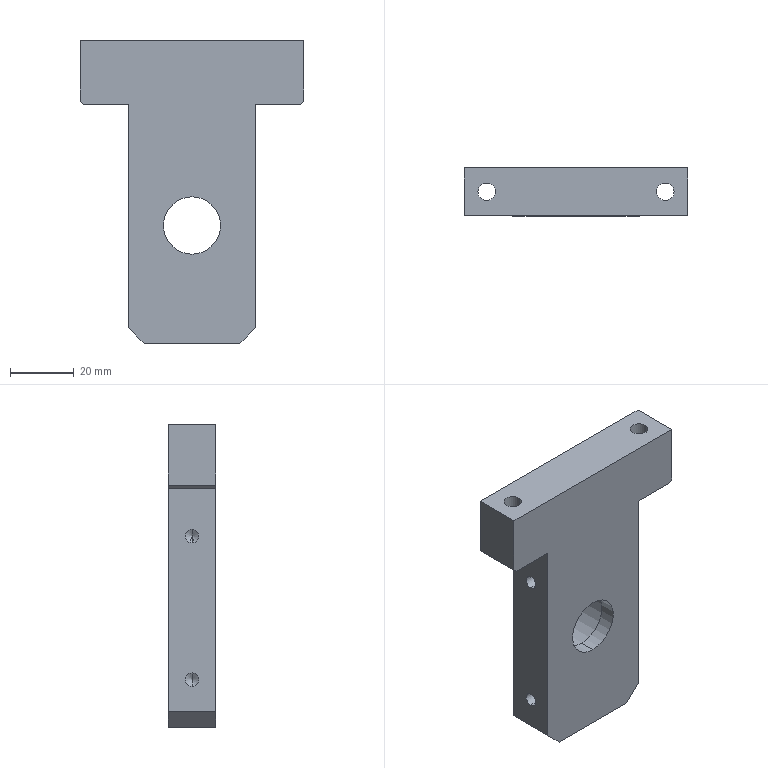Part | SolidWorks | features BaseBody 1 | 1 solid | 45 faces | box 70 x 15 x 95 mm | volume 57528 mm3 | cylinder 20 | plane 17 | cone 8 | commonest cylinder face diameters 4.2 x8 5.5 x4 10 x4 18 x2 24 x2
STEP:
#1=CARTESIAN_POINT('',(-10.345,7.5,-15.013));
#2=VERTEX_POINT('',#1);
#3=CARTESIAN_POINT('',(-10.345,7.5,-10.813));
#4=VERTEX_POINT('',#3);
#5=CARTESIAN_POINT('',(-10.345,7.5,-12.913));
#6=DIRECTION('',(-1.,0.,0.));
#7=DIRECTION('',(0.,0.,1.));
#8=AXIS2_PLACEMENT_3D('',#5,#6,#7);
#9=CIRCLE('',#8,2.1);
#10=EDGE_CURVE('',#2,#4,#9,.T.);
#11=ORIENTED_EDGE('',*,*,#10,.F.);
#12=CARTESIAN_POINT('',(-22.745,7.5,-15.013));
#13=VERTEX_POINT('',#12);
#14=CARTESIAN_POINT('',(-22.745,7.5,-15.013));
#15=DIRECTION('',(-1.,0.,0.));
#16=VECTOR('',#15,1000.);
#17=LINE('',#14,#16);
#18=EDGE_CURVE('',#2,#13,#17,.T.);
#19=ORIENTED_EDGE('',*,*,#18,.T.);
#20=CARTESIAN_POINT('',(-22.745,7.5,-10.813));
#21=VERTEX_POINT('',#20);
#22=CARTESIAN_POINT('',(-22.745,7.5,-12.913));
#23=DIRECTION('',(-1.,0.,0.));
#24=DIRECTION('',(0.,0.,1.));
#25=AXIS2_PLACEMENT_3D('',#22,#23,#24);
#26=CIRCLE('',#25,2.1);
#27=EDGE_CURVE('',#13,#21,#26,.T.);
#28=ORIENTED_EDGE('',*,*,#27,.T.);
#29=CARTESIAN_POINT('',(-22.745,7.5,-10.813));
#30=DIRECTION('',(-1.,0.,0.));
#31=VECTOR('',#30,1000.);
#32=LINE('',#29,#31);
#33=EDGE_CURVE('',#4,#21,#32,.T.);
#34=ORIENTED_EDGE('',*,*,#33,.F.);
#35=EDGE_LOOP('',(#11,#19,#28,#34));
#36=FACE_OUTER_BOUND('',#35,.T.);
#37=CARTESIAN_POINT('',(-22.745,7.5,-12.913));
#38=DIRECTION('',(-1.,0.,0.));
#39=DIRECTION('',(0.,0.,1.));
#40=AXIS2_PLACEMENT_3D('',#37,#38,#39);
#41=CYLINDRICAL_SURFACE('',#40,2.1);
#42=ADVANCED_FACE('',(#36),#41,.F.);
#43=CARTESIAN_POINT('',(-9.083,7.5,-12.913));
#44=VERTEX_POINT('',#43);
#45=CARTESIAN_POINT('',(-10.345,7.5,-10.813));
#46=DIRECTION('',(-0.515,0.,0.8572));
#47=VECTOR('',#46,1000.);
#48=LINE('',#45,#47);
#49=EDGE_CURVE('',#44,#4,#48,.T.);
#50=ORIENTED_EDGE('',*,*,#49,.F.);
#51=CARTESIAN_POINT('',(-10.345,7.5,-15.013));
#52=DIRECTION('',(-0.515,0.,-0.8572));
#53=VECTOR('',#52,1000.);
#54=LINE('',#51,#53);
#55=EDGE_CURVE('',#44,#2,#54,.T.);
#56=ORIENTED_EDGE('',*,*,#55,.T.);
#57=ORIENTED_EDGE('',*,*,#10,.T.);
#58=EDGE_LOOP('',(#50,#56,#57));
#59=FACE_OUTER_BOUND('',#58,.T.);
#60=CARTESIAN_POINT('',(-10.345,7.5,-12.913));
#61=DIRECTION('',(-1.,0.,0.));
#62=DIRECTION('',(0.,0.,1.));
#63=AXIS2_PLACEMENT_3D('',#60,#61,#62);
#64=CONICAL_SURFACE('',#63,2.1,1.03);
#65=ADVANCED_FACE('',(#59),#64,.F.);
#66=CARTESIAN_POINT('',(-10.345,7.5,29.987));
#67=VERTEX_POINT('',#66);
#68=CARTESIAN_POINT('',(-10.345,7.5,34.187));
#69=VERTEX_POINT('',#68);
#70=CARTESIAN_POINT('',(-10.345,7.5,32.087));
#71=DIRECTION('',(-1.,0.,0.));
#72=DIRECTION('',(0.,0.,1.));
#73=AXIS2_PLACEMENT_3D('',#70,#71,#72);
#74=CIRCLE('',#73,2.1);
#75=EDGE_CURVE('',#67,#69,#74,.T.);
#76=ORIENTED_EDGE('',*,*,#75,.F.);
#77=CARTESIAN_POINT('',(-22.745,7.5,29.987));
#78=VERTEX_POINT('',#77);
#79=CARTESIAN_POINT('',(-22.745,7.5,29.987));
#80=DIRECTION('',(-1.,0.,0.));
#81=VECTOR('',#80,1000.);
#82=LINE('',#79,#81);
#83=EDGE_CURVE('',#67,#78,#82,.T.);
#84=ORIENTED_EDGE('',*,*,#83,.T.);
#85=CARTESIAN_POINT('',(-22.745,7.5,34.187));
#86=VERTEX_POINT('',#85);
#87=CARTESIAN_POINT('',(-22.745,7.5,32.087));
#88=DIRECTION('',(-1.,0.,0.));
#89=DIRECTION('',(0.,0.,1.));
#90=AXIS2_PLACEMENT_3D('',#87,#88,#89);
#91=CIRCLE('',#90,2.1);
#92=EDGE_CURVE('',#78,#86,#91,.T.);
#93=ORIENTED_EDGE('',*,*,#92,.T.);
#94=CARTESIAN_POINT('',(-22.745,7.5,34.187));
#95=DIRECTION('',(-1.,0.,0.));
#96=VECTOR('',#95,1000.);
#97=LINE('',#94,#96);
#98=EDGE_CURVE('',#69,#86,#97,.T.);
#99=ORIENTED_EDGE('',*,*,#98,.F.);
#100=EDGE_LOOP('',(#76,#84,#93,#99));
#101=FACE_OUTER_BOUND('',#100,.T.);
#102=CARTESIAN_POINT('',(-22.745,7.5,32.087));
#103=DIRECTION('',(-1.,0.,0.));
#104=DIRECTION('',(0.,0.,1.));
#105=AXIS2_PLACEMENT_3D('',#102,#103,#104);
#106=CYLINDRICAL_SURFACE('',#105,2.1);
#107=ADVANCED_FACE('',(#101),#106,.F.);
#108=CARTESIAN_POINT('',(-9.083,7.5,32.087));
#109=VERTEX_POINT('',#108);
#110=CARTESIAN_POINT('',(-10.345,7.5,34.187));
#111=DIRECTION('',(-0.515,0.,0.8572));
#112=VECTOR('',#111,1000.);
#113=LINE('',#110,#112);
#114=EDGE_CURVE('',#109,#69,#113,.T.);
#115=ORIENTED_EDGE('',*,*,#114,.F.);
#116=CARTESIAN_POINT('',(-10.345,7.5,29.987));
#117=DIRECTION('',(-0.515,0.,-0.8572));
#118=VECTOR('',#117,1000.);
#119=LINE('',#116,#118);
#120=EDGE_CURVE('',#109,#67,#119,.T.);
#121=ORIENTED_EDGE('',*,*,#120,.T.);
#122=ORIENTED_EDGE('',*,*,#75,.T.);
#123=EDGE_LOOP('',(#115,#121,#122));
#124=FACE_OUTER_BOUND('',#123,.T.);
#125=CARTESIAN_POINT('',(-10.345,7.5,32.087));
#126=DIRECTION('',(-1.,0.,0.));
#127=DIRECTION('',(0.,0.,1.));
#128=AXIS2_PLACEMENT_3D('',#125,#126,#127);
#129=CONICAL_SURFACE('',#128,2.1,1.03);
#130=ADVANCED_FACE('',(#124),#129,.F.);
#131=CARTESIAN_POINT('',(4.855,7.5,-10.813));
#132=VERTEX_POINT('',#131);
#133=CARTESIAN_POINT('',(4.855,7.5,-15.013));
#134=VERTEX_POINT('',#133);
#135=CARTESIAN_POINT('',(4.855,7.5,-12.913));
#136=DIRECTION('',(1.,0.,0.));
#137=DIRECTION('',(0.,0.,-1.));
#138=AXIS2_PLACEMENT_3D('',#135,#136,#137);
#139=CIRCLE('',#138,2.1);
#140=EDGE_CURVE('',#132,#134,#139,.T.);
#141=ORIENTED_EDGE('',*,*,#140,.F.);
#142=CARTESIAN_POINT('',(17.255,7.5,-10.813));
#143=VERTEX_POINT('',#142);
#144=CARTESIAN_POINT('',(17.255,7.5,-10.813));
#145=DIRECTION('',(1.,0.,0.));
#146=VECTOR('',#145,1000.);
#147=LINE('',#144,#146);
#148=EDGE_CURVE('',#132,#143,#147,.T.);
#149=ORIENTED_EDGE('',*,*,#148,.T.);
#150=CARTESIAN_POINT('',(17.255,7.5,-15.013));
#151=VERTEX_POINT('',#150);
#152=CARTESIAN_POINT('',(17.255,7.5,-12.913));
#153=DIRECTION('',(1.,0.,0.));
#154=DIRECTION('',(0.,0.,-1.));
#155=AXIS2_PLACEMENT_3D('',#152,#153,#154);
#156=CIRCLE('',#155,2.1);
#157=EDGE_CURVE('',#143,#151,#156,.T.);
#158=ORIENTED_EDGE('',*,*,#157,.T.);
#159=CARTESIAN_POINT('',(17.255,7.5,-15.013));
#160=DIRECTION('',(1.,0.,0.));
#161=VECTOR('',#160,1000.);
#162=LINE('',#159,#161);
#163=EDGE_CURVE('',#134,#151,#162,.T.);
#164=ORIENTED_EDGE('',*,*,#163,.F.);
#165=EDGE_LOOP('',(#141,#149,#158,#164));
#166=FACE_OUTER_BOUND('',#165,.T.);
#167=CARTESIAN_POINT('',(17.255,7.5,-12.913));
#168=DIRECTION('',(1.,0.,0.));
#169=DIRECTION('',(0.,0.,-1.));
#170=AXIS2_PLACEMENT_3D('',#167,#168,#169);
#171=CYLINDRICAL_SURFACE('',#170,2.1);
#172=ADVANCED_FACE('',(#166),#171,.F.);
#173=CARTESIAN_POINT('',(3.593,7.5,-12.913));
#174=VERTEX_POINT('',#173);
#175=CARTESIAN_POINT('',(4.855,7.5,-15.013));
#176=DIRECTION('',(0.515,0.,-0.8572));
#177=VECTOR('',#176,1000.);
#178=LINE('',#175,#177);
#179=EDGE_CURVE('',#174,#134,#178,.T.);
#180=ORIENTED_EDGE('',*,*,#179,.F.);
#181=CARTESIAN_POINT('',(4.855,7.5,-10.813));
#182=DIRECTION('',(0.515,0.,0.8572));
#183=VECTOR('',#182,1000.);
#184=LINE('',#181,#183);
#185=EDGE_CURVE('',#174,#132,#184,.T.);
#186=ORIENTED_EDGE('',*,*,#185,.T.);
#187=ORIENTED_EDGE('',*,*,#140,.T.);
#188=EDGE_LOOP('',(#180,#186,#187));
#189=FACE_OUTER_BOUND('',#188,.T.);
#190=CARTESIAN_POINT('',(4.855,7.5,-12.913));
#191=DIRECTION('',(1.,0.,0.));
#192=DIRECTION('',(0.,0.,-1.));
#193=AXIS2_PLACEMENT_3D('',#190,#191,#192);
#194=CONICAL_SURFACE('',#193,2.1,1.03);
#195=ADVANCED_FACE('',(#189),#194,.F.);
#196=CARTESIAN_POINT('',(4.855,7.5,34.187));
#197=VERTEX_POINT('',#196);
#198=CARTESIAN_POINT('',(4.855,7.5,29.987));
#199=VERTEX_POINT('',#198);
#200=CARTESIAN_POINT('',(4.855,7.5,32.087));
#201=DIRECTION('',(1.,0.,0.));
#202=DIRECTION('',(0.,0.,-1.));
#203=AXIS2_PLACEMENT_3D('',#200,#201,#202);
#204=CIRCLE('',#203,2.1);
#205=EDGE_CURVE('',#197,#199,#204,.T.);
#206=ORIENTED_EDGE('',*,*,#205,.F.);
#207=CARTESIAN_POINT('',(17.255,7.5,34.187));
#208=VERTEX_POINT('',#207);
#209=CARTESIAN_POINT('',(17.255,7.5,34.187));
#210=DIRECTION('',(1.,0.,0.));
#211=VECTOR('',#210,1000.);
#212=LINE('',#209,#211);
#213=EDGE_CURVE('',#197,#208,#212,.T.);
#214=ORIENTED_EDGE('',*,*,#213,.T.);
#215=CARTESIAN_POINT('',(17.255,7.5,29.987));
#216=VERTEX_POINT('',#215);
#217=CARTESIAN_POINT('',(17.255,7.5,32.087));
#218=DIRECTION('',(1.,0.,0.));
#219=DIRECTION('',(0.,0.,-1.));
#220=AXIS2_PLACEMENT_3D('',#217,#218,#219);
#221=CIRCLE('',#220,2.1);
#222=EDGE_CURVE('',#208,#216,#221,.T.);
#223=ORIENTED_EDGE('',*,*,#222,.T.);
#224=CARTESIAN_POINT('',(17.255,7.5,29.987));
#225=DIRECTION('',(1.,0.,0.));
#226=VECTOR('',#225,1000.);
#227=LINE('',#224,#226);
#228=EDGE_CURVE('',#199,#216,#227,.T.);
#229=ORIENTED_EDGE('',*,*,#228,.F.);
#230=EDGE_LOOP('',(#206,#214,#223,#229));
#231=FACE_OUTER_BOUND('',#230,.T.);
#232=CARTESIAN_POINT('',(17.255,7.5,32.087));
#233=DIRECTION('',(1.,0.,0.));
#234=DIRECTION('',(0.,0.,-1.));
#235=AXIS2_PLACEMENT_3D('',#232,#233,#234);
#236=CYLINDRICAL_SURFACE('',#235,2.1);
#237=ADVANCED_FACE('',(#231),#236,.F.);
#238=CARTESIAN_POINT('',(3.593,7.5,32.087));
#239=VERTEX_POINT('',#238);
#240=CARTESIAN_POINT('',(4.855,7.5,29.987));
#241=DIRECTION('',(0.515,0.,-0.8572));
#242=VECTOR('',#241,1000.);
#243=LINE('',#240,#242);
#244=EDGE_CURVE('',#239,#199,#243,.T.);
#245=ORIENTED_EDGE('',*,*,#244,.F.);
#246=CARTESIAN_POINT('',(4.855,7.5,34.187));
#247=DIRECTION('',(0.515,0.,0.8572));
#248=VECTOR('',#247,1000.);
#249=LINE('',#246,#248);
#250=EDGE_CURVE('',#239,#197,#249,.T.);
#251=ORIENTED_EDGE('',*,*,#250,.T.);
#252=ORIENTED_EDGE('',*,*,#205,.T.);
#253=EDGE_LOOP('',(#245,#251,#252));
#254=FACE_OUTER_BOUND('',#253,.T.);
#255=CARTESIAN_POINT('',(4.855,7.5,32.087));
#256=DIRECTION('',(1.,0.,0.));
#257=DIRECTION('',(0.,0.,-1.));
#258=AXIS2_PLACEMENT_3D('',#255,#256,#257);
#259=CONICAL_SURFACE('',#258,2.1,1.03);
#260=ADVANCED_FACE('',(#254),#259,.F.);
#261=CARTESIAN_POINT('',(30.255,7.5,52.787));
#262=VERTEX_POINT('',#261);
#263=CARTESIAN_POINT('',(20.255,7.5,52.787));
#264=VERTEX_POINT('',#263);
#265=CARTESIAN_POINT('',(25.255,7.5,52.787));
#266=DIRECTION('',(0.,0.,-1.));
#267=DIRECTION('',(-1.,0.,0.));
#268=AXIS2_PLACEMENT_3D('',#265,#266,#267);
#269=CIRCLE('',#268,5.);
#270=EDGE_CURVE('',#262,#264,#269,.T.);
#271=ORIENTED_EDGE('',*,*,#270,.F.);
#272=CARTESIAN_POINT('',(30.255,7.5,47.087));
#273=VERTEX_POINT('',#272);
#274=CARTESIAN_POINT('',(30.255,7.5,47.087));
#275=DIRECTION('',(0.,0.,-1.));
#276=VECTOR('',#275,1000.);
#277=LINE('',#274,#276);
#278=EDGE_CURVE('',#262,#273,#277,.T.);
#279=ORIENTED_EDGE('',*,*,#278,.T.);
#280=CARTESIAN_POINT('',(20.255,7.5,47.087));
#281=VERTEX_POINT('',#280);
#282=CARTESIAN_POINT('',(25.255,7.5,47.087));
#283=DIRECTION('',(0.,0.,-1.));
#284=DIRECTION('',(-1.,0.,0.));
#285=AXIS2_PLACEMENT_3D('',#282,#283,#284);
#286=CIRCLE('',#285,5.);
#287=EDGE_CURVE('',#273,#281,#286,.T.);
#288=ORIENTED_EDGE('',*,*,#287,.T.);
#289=CARTESIAN_POINT('',(20.255,7.5,47.087));
#290=DIRECTION('',(0.,0.,-1.));
#291=VECTOR('',#290,1000.);
#292=LINE('',#289,#291);
#293=EDGE_CURVE('',#264,#281,#292,.T.);
#294=ORIENTED_EDGE('',*,*,#293,.F.);
#295=EDGE_LOOP('',(#271,#279,#288,#294));
#296=FACE_OUTER_BOUND('',#295,.T.);
#297=CARTESIAN_POINT('',(25.255,7.5,47.087));
#298=DIRECTION('',(0.,0.,-1.));
#299=DIRECTION('',(-1.,0.,0.));
#300=AXIS2_PLACEMENT_3D('',#297,#298,#299);
#301=CYLINDRICAL_SURFACE('',#300,5.);
#302=ADVANCED_FACE('',(#296),#301,.F.);
#303=CARTESIAN_POINT('',(28.005,7.5,67.087));
#304=VERTEX_POINT('',#303);
#305=CARTESIAN_POINT('',(22.505,7.5,67.087));
#306=VERTEX_POINT('',#305);
#307=CARTESIAN_POINT('',(25.255,7.5,67.087));
#308=DIRECTION('',(0.,0.,-1.));
#309=DIRECTION('',(-1.,0.,0.));
#310=AXIS2_PLACEMENT_3D('',#307,#308,#309);
#311=CIRCLE('',#310,2.75);
#312=EDGE_CURVE('',#304,#306,#311,.T.);
#313=ORIENTED_EDGE('',*,*,#312,.F.);
#314=CARTESIAN_POINT('',(28.005,7.5,52.787));
#315=VERTEX_POINT('',#314);
#316=CARTESIAN_POINT('',(28.005,7.5,47.087));
#317=DIRECTION('',(0.,0.,-1.));
#318=VECTOR('',#317,1000.);
#319=LINE('',#316,#318);
#320=EDGE_CURVE('',#304,#315,#319,.T.);
#321=ORIENTED_EDGE('',*,*,#320,.T.);
#322=CARTESIAN_POINT('',(22.505,7.5,52.787));
#323=VERTEX_POINT('',#322);
#324=CARTESIAN_POINT('',(25.255,7.5,52.787));
#325=DIRECTION('',(0.,0.,-1.));
#326=DIRECTION('',(-1.,0.,0.));
#327=AXIS2_PLACEMENT_3D('',#324,#325,#326);
#328=CIRCLE('',#327,2.75);
#329=EDGE_CURVE('',#315,#323,#328,.T.);
#330=ORIENTED_EDGE('',*,*,#329,.T.);
#331=CARTESIAN_POINT('',(22.505,7.5,47.087));
#332=DIRECTION('',(0.,0.,-1.));
#333=VECTOR('',#332,1000.);
#334=LINE('',#331,#333);
#335=EDGE_CURVE('',#306,#323,#334,.T.);
#336=ORIENTED_EDGE('',*,*,#335,.F.);
#337=EDGE_LOOP('',(#313,#321,#330,#336));
#338=FACE_OUTER_BOUND('',#337,.T.);
#339=CARTESIAN_POINT('',(25.255,7.5,47.087));
#340=DIRECTION('',(0.,0.,-1.));
#341=DIRECTION('',(-1.,0.,0.));
#342=AXIS2_PLACEMENT_3D('',#339,#340,#341);
#343=CYLINDRICAL_SURFACE('',#342,2.75);
#344=ADVANCED_FACE('',(#338),#343,.F.);
#345=CARTESIAN_POINT('',(-25.745,7.5,52.787));
#346=VERTEX_POINT('',#345);
#347=CARTESIAN_POINT('',(-35.745,7.5,52.787));
#348=VERTEX_POINT('',#347);
#349=CARTESIAN_POINT('',(-30.745,7.5,52.787));
#350=DIRECTION('',(0.,0.,-1.));
#351=DIRECTION('',(-1.,0.,0.));
#352=AXIS2_PLACEMENT_3D('',#349,#350,#351);
#353=CIRCLE('',#352,5.);
#354=EDGE_CURVE('',#346,#348,#353,.T.);
#355=ORIENTED_EDGE('',*,*,#354,.F.);
#356=CARTESIAN_POINT('',(-25.745,7.5,47.087));
#357=VERTEX_POINT('',#356);
#358=CARTESIAN_POINT('',(-25.745,7.5,47.087));
#359=DIRECTION('',(0.,0.,-1.));
#360=VECTOR('',#359,1000.);
#361=LINE('',#358,#360);
#362=EDGE_CURVE('',#346,#357,#361,.T.);
#363=ORIENTED_EDGE('',*,*,#362,.T.);
#364=CARTESIAN_POINT('',(-35.745,7.5,47.087));
#365=VERTEX_POINT('',#364);
#366=CARTESIAN_POINT('',(-30.745,7.5,47.087));
#367=DIRECTION('',(0.,0.,-1.));
#368=DIRECTION('',(-1.,0.,0.));
#369=AXIS2_PLACEMENT_3D('',#366,#367,#368);
#370=CIRCLE('',#369,5.);
#371=EDGE_CURVE('',#357,#365,#370,.T.);
#372=ORIENTED_EDGE('',*,*,#371,.T.);
#373=CARTESIAN_POINT('',(-35.745,7.5,47.087));
#374=DIRECTION('',(0.,0.,-1.));
#375=VECTOR('',#374,1000.);
#376=LINE('',#373,#375);
#377=EDGE_CURVE('',#348,#365,#376,.T.);
#378=ORIENTED_EDGE('',*,*,#377,.F.);
#379=EDGE_LOOP('',(#355,#363,#372,#378));
#380=FACE_OUTER_BOUND('',#379,.T.);
#381=CARTESIAN_POINT('',(-30.745,7.5,47.087));
#382=DIRECTION('',(0.,0.,-1.));
#383=DIRECTION('',(-1.,0.,0.));
#384=AXIS2_PLACEMENT_3D('',#381,#382,#383);
#385=CYLINDRICAL_SURFACE('',#384,5.);
#386=ADVANCED_FACE('',(#380),#385,.F.);
#387=CARTESIAN_POINT('',(-27.995,7.5,67.087));
#388=VERTEX_POINT('',#387);
#389=CARTESIAN_POINT('',(-33.495,7.5,67.087));
#390=VERTEX_POINT('',#389);
#391=CARTESIAN_POINT('',(-30.745,7.5,67.087));
#392=DIRECTION('',(0.,0.,-1.));
#393=DIRECTION('',(-1.,0.,0.));
#394=AXIS2_PLACEMENT_3D('',#391,#392,#393);
#395=CIRCLE('',#394,2.75);
#396=EDGE_CURVE('',#388,#390,#395,.T.);
#397=ORIENTED_EDGE('',*,*,#396,.F.);
#398=CARTESIAN_POINT('',(-27.995,7.5,52.787));
#399=VERTEX_POINT('',#398);
#400=CARTESIAN_POINT('',(-27.995,7.5,47.087));
#401=DIRECTION('',(0.,0.,-1.));
#402=VECTOR('',#401,1000.);
#403=LINE('',#400,#402);
#404=EDGE_CURVE('',#388,#399,#403,.T.);
#405=ORIENTED_EDGE('',*,*,#404,.T.);
#406=CARTESIAN_POINT('',(-33.495,7.5,52.787));
#407=VERTEX_POINT('',#406);
#408=CARTESIAN_POINT('',(-30.745,7.5,52.787));
#409=DIRECTION('',(0.,0.,-1.));
#410=DIRECTION('',(-1.,0.,0.));
#411=AXIS2_PLACEMENT_3D('',#408,#409,#410);
#412=CIRCLE('',#411,2.75);
#413=EDGE_CURVE('',#399,#407,#412,.T.);
#414=ORIENTED_EDGE('',*,*,#413,.T.);
#415=CARTESIAN_POINT('',(-33.495,7.5,47.087));
#416=DIRECTION('',(0.,0.,-1.));
#417=VECTOR('',#416,1000.);
#418=LINE('',#415,#417);
#419=EDGE_CURVE('',#390,#407,#418,.T.);
#420=ORIENTED_EDGE('',*,*,#419,.F.);
#421=EDGE_LOOP('',(#397,#405,#414,#420));
#422=FACE_OUTER_BOUND('',#421,.T.);
#423=CARTESIAN_POINT('',(-30.745,7.5,47.087));
#424=DIRECTION('',(0.,0.,-1.));
#425=DIRECTION('',(-1.,0.,0.));
#426=AXIS2_PLACEMENT_3D('',#423,#424,#425);
#427=CYLINDRICAL_SURFACE('',#426,2.75);
#428=ADVANCED_FACE('',(#422),#427,.F.);
#429=CARTESIAN_POINT('',(-2.745,5.,-2.913));
#430=VERTEX_POINT('',#429);
#431=CARTESIAN_POINT('',(-2.745,5.,21.087));
#432=VERTEX_POINT('',#431);
#433=CARTESIAN_POINT('',(-2.745,5.,9.087));
#434=DIRECTION('',(0.,1.,0.));
#435=DIRECTION('',(0.,0.,1.));
#436=AXIS2_PLACEMENT_3D('',#433,#434,#435);
#437=CIRCLE('',#436,12.);
#438=EDGE_CURVE('',#430,#432,#437,.T.);
#439=ORIENTED_EDGE('',*,*,#438,.F.);
#440=CARTESIAN_POINT('',(-2.745,15.,-2.913));
#441=VERTEX_POINT('',#440);
#442=CARTESIAN_POINT('',(-2.745,5.,-2.913));
#443=DIRECTION('',(0.,1.,0.));
#444=VECTOR('',#443,1000.);
#445=LINE('',#442,#444);
#446=EDGE_CURVE('',#430,#441,#445,.T.);
#447=ORIENTED_EDGE('',*,*,#446,.T.);
#448=CARTESIAN_POINT('',(-2.745,15.,21.087));
#449=VERTEX_POINT('',#448);
#450=CARTESIAN_POINT('',(-2.745,15.,9.087));
#451=DIRECTION('',(0.,1.,0.));
#452=DIRECTION('',(0.,0.,1.));
#453=AXIS2_PLACEMENT_3D('',#450,#451,#452);
#454=CIRCLE('',#453,12.);
#455=EDGE_CURVE('',#441,#449,#454,.T.);
#456=ORIENTED_EDGE('',*,*,#455,.T.);
#457=CARTESIAN_POINT('',(-2.745,5.,21.087));
#458=DIRECTION('',(0.,1.,0.));
#459=VECTOR('',#458,1000.);
#460=LINE('',#457,#459);
#461=EDGE_CURVE('',#432,#449,#460,.T.);
#462=ORIENTED_EDGE('',*,*,#461,.F.);
#463=EDGE_LOOP('',(#439,#447,#456,#462));
#464=FACE_OUTER_BOUND('',#463,.T.);
#465=CARTESIAN_POINT('',(-2.745,5.,9.087));
#466=DIRECTION('',(0.,1.,0.));
#467=DIRECTION('',(0.,0.,1.));
#468=AXIS2_PLACEMENT_3D('',#465,#466,#467);
#469=CYLINDRICAL_SURFACE('',#468,12.);
#470=ADVANCED_FACE('',(#464),#469,.F.);
#471=CARTESIAN_POINT('',(-2.745,5.,0.08706));
#472=VERTEX_POINT('',#471);
#473=CARTESIAN_POINT('',(-2.745,5.,18.087));
#474=VERTEX_POINT('',#473);
#475=CARTESIAN_POINT('',(-2.745,5.,9.087));
#476=DIRECTION('',(0.,1.,0.));
#477=DIRECTION('',(0.,0.,1.));
#478=AXIS2_PLACEMENT_3D('',#475,#476,#477);
#479=CIRCLE('',#478,9.);
#480=EDGE_CURVE('',#472,#474,#479,.T.);
#481=ORIENTED_EDGE('',*,*,#480,.T.);
#482=CARTESIAN_POINT('',(-2.745,0.,18.087));
#483=VERTEX_POINT('',#482);
#484=CARTESIAN_POINT('',(-2.745,15.,18.087));
#485=DIRECTION('',(0.,-1.,0.));
#486=VECTOR('',#485,1000.);
#487=LINE('',#484,#486);
#488=EDGE_CURVE('',#474,#483,#487,.T.);
#489=ORIENTED_EDGE('',*,*,#488,.T.);
#490=CARTESIAN_POINT('',(-2.745,0.,0.08706));
#491=VERTEX_POINT('',#490);
#492=CARTESIAN_POINT('',(-2.745,0.,9.087));
#493=DIRECTION('',(0.,1.,0.));
#494=DIRECTION('',(0.,0.,1.));
#495=AXIS2_PLACEMENT_3D('',#492,#493,#494);
#496=CIRCLE('',#495,9.);
#497=EDGE_CURVE('',#491,#483,#496,.T.);
#498=ORIENTED_EDGE('',*,*,#497,.F.);
#499=CARTESIAN_POINT('',(-2.745,15.,0.08706));
#500=DIRECTION('',(0.,-1.,0.));
#501=VECTOR('',#500,1000.);
#502=LINE('',#499,#501);
#503=EDGE_CURVE('',#472,#491,#502,.T.);
#504=ORIENTED_EDGE('',*,*,#503,.F.);
#505=EDGE_LOOP('',(#481,#489,#498,#504));
#506=FACE_OUTER_BOUND('',#505,.T.);
#507=CARTESIAN_POINT('',(-2.745,15.,9.087));
#508=DIRECTION('',(0.,-1.,0.));
#509=DIRECTION('',(0.,0.,-1.));
#510=AXIS2_PLACEMENT_3D('',#507,#508,#509);
#511=CYLINDRICAL_SURFACE('',#510,9.);
#512=ADVANCED_FACE('',(#506),#511,.F.);
#513=CARTESIAN_POINT('',(25.255,7.5,52.787));
#514=DIRECTION('',(0.,0.,-1.));
#515=DIRECTION('',(-1.,0.,0.));
#516=AXIS2_PLACEMENT_3D('',#513,#514,#515);
#517=CIRCLE('',#516,2.75);
#518=EDGE_CURVE('',#323,#315,#517,.T.);
#519=ORIENTED_EDGE('',*,*,#518,.F.);
#520=ORIENTED_EDGE('',*,*,#329,.F.);
#521=EDGE_LOOP('',(#519,#520));
#522=FACE_BOUND('',#521,.T.);
#523=CARTESIAN_POINT('',(25.255,7.5,52.787));
#524=DIRECTION('',(0.,0.,-1.));
#525=DIRECTION('',(-1.,0.,0.));
#526=AXIS2_PLACEMENT_3D('',#523,#524,#525);
#527=CIRCLE('',#526,5.);
#528=EDGE_CURVE('',#264,#262,#527,.T.);
#529=ORIENTED_EDGE('',*,*,#528,.T.);
#530=ORIENTED_EDGE('',*,*,#270,.T.);
#531=EDGE_LOOP('',(#529,#530));
#532=FACE_OUTER_BOUND('',#531,.T.);
#533=CARTESIAN_POINT('',(28.005,7.5,52.787));
#534=DIRECTION('',(0.,0.,1.));
#535=DIRECTION('',(1.,0.,0.));
#536=AXIS2_PLACEMENT_3D('',#533,#534,#535);
#537=PLANE('',#536);
#538=ADVANCED_FACE('',(#522,#532),#537,.F.);
#539=CARTESIAN_POINT('',(-30.745,7.5,52.787));
#540=DIRECTION('',(0.,0.,-1.));
#541=DIRECTION('',(-1.,0.,0.));
#542=AXIS2_PLACEMENT_3D('',#539,#540,#541);
#543=CIRCLE('',#542,2.75);
#544=EDGE_CURVE('',#407,#399,#543,.T.);
#545=ORIENTED_EDGE('',*,*,#544,.F.);
#546=ORIENTED_EDGE('',*,*,#413,.F.);
#547=EDGE_LOOP('',(#545,#546));
#548=FACE_BOUND('',#547,.T.);
#549=CARTESIAN_POINT('',(-30.745,7.5,52.787));
#550=DIRECTION('',(0.,0.,-1.));
#551=DIRECTION('',(-1.,0.,0.));
#552=AXIS2_PLACEMENT_3D('',#549,#550,#551);
#553=CIRCLE('',#552,5.);
#554=EDGE_CURVE('',#348,#346,#553,.T.);
#555=ORIENTED_EDGE('',*,*,#554,.T.);
#556=ORIENTED_EDGE('',*,*,#354,.T.);
#557=EDGE_LOOP('',(#555,#556));
#558=FACE_OUTER_BOUND('',#557,.T.);
#559=CARTESIAN_POINT('',(-27.995,7.5,52.787));
#560=DIRECTION('',(0.,0.,1.));
#561=DIRECTION('',(1.,0.,0.));
#562=AXIS2_PLACEMENT_3D('',#559,#560,#561);
#563=PLANE('',#562);
#564=ADVANCED_FACE('',(#548,#558),#563,.F.);
#565=CARTESIAN_POINT('',(-36.745,15.,47.087));
#566=VERTEX_POINT('',#565);
#567=CARTESIAN_POINT('',(-37.745,15.,48.087));
#568=VERTEX_POINT('',#567);
#569=CARTESIAN_POINT('',(5.171,15.,5.171));
#570=DIRECTION('',(-0.7071,0.,0.7071));
#571=VECTOR('',#570,1000.);
#572=LINE('',#569,#571);
#573=EDGE_CURVE('',#566,#568,#572,.T.);
#574=ORIENTED_EDGE('',*,*,#573,.F.);
#575=CARTESIAN_POINT('',(-36.745,0.,47.087));
#576=VERTEX_POINT('',#575);
#577=CARTESIAN_POINT('',(-36.745,15.,47.087));
#578=DIRECTION('',(0.,1.,0.));
#579=VECTOR('',#578,1000.);
#580=LINE('',#577,#579);
#581=EDGE_CURVE('',#576,#566,#580,.T.);
#582=ORIENTED_EDGE('',*,*,#581,.F.);
#583=CARTESIAN_POINT('',(-37.745,0.,48.087));
#584=VERTEX_POINT('',#583);
#585=CARTESIAN_POINT('',(-37.745,0.,48.087));
#586=DIRECTION('',(0.7071,0.,-0.7071));
#587=VECTOR('',#586,1000.);
#588=LINE('',#585,#587);
#589=EDGE_CURVE('',#584,#576,#588,.T.);
#590=ORIENTED_EDGE('',*,*,#589,.F.);
#591=CARTESIAN_POINT('',(-37.745,15.,48.087));
#592=DIRECTION('',(0.,-1.,0.));
#593=VECTOR('',#592,1000.);
#594=LINE('',#591,#593);
#595=EDGE_CURVE('',#568,#584,#594,.T.);
#596=ORIENTED_EDGE('',*,*,#595,.F.);
#597=EDGE_LOOP('',(#574,#582,#590,#596));
#598=FACE_OUTER_BOUND('',#597,.T.);
#599=CARTESIAN_POINT('',(-37.745,15.,48.087));
#600=DIRECTION('',(0.7071,0.,0.7071));
#601=DIRECTION('',(0.,-1.,0.));
#602=AXIS2_PLACEMENT_3D('',#599,#600,#601);
#603=PLANE('',#602);
#604=ADVANCED_FACE('',(#598),#603,.F.);
#605=CARTESIAN_POINT('',(32.255,15.,48.087));
#606=VERTEX_POINT('',#605);
#607=CARTESIAN_POINT('',(31.255,15.,47.087));
#608=VERTEX_POINT('',#607);
#609=CARTESIAN_POINT('',(-7.916,15.,7.916));
#610=DIRECTION('',(-0.7071,0.,-0.7071));
#611=VECTOR('',#610,1000.);
#612=LINE('',#609,#611);
#613=EDGE_CURVE('',#606,#608,#612,.T.);
#614=ORIENTED_EDGE('',*,*,#613,.F.);
#615=CARTESIAN_POINT('',(32.255,0.,48.087));
#616=VERTEX_POINT('',#615);
#617=CARTESIAN_POINT('',(32.255,15.,48.087));
#618=DIRECTION('',(0.,1.,0.));
#619=VECTOR('',#618,1000.);
#620=LINE('',#617,#619);
#621=EDGE_CURVE('',#616,#606,#620,.T.);
#622=ORIENTED_EDGE('',*,*,#621,.F.);
#623=CARTESIAN_POINT('',(31.255,0.,47.087));
#624=VERTEX_POINT('',#623);
#625=CARTESIAN_POINT('',(31.255,0.,47.087));
#626=DIRECTION('',(0.7071,0.,0.7071));
#627=VECTOR('',#626,1000.);
#628=LINE('',#625,#627);
#629=EDGE_CURVE('',#624,#616,#628,.T.);
#630=ORIENTED_EDGE('',*,*,#629,.F.);
#631=CARTESIAN_POINT('',(31.255,15.,47.087));
#632=DIRECTION('',(0.,-1.,0.));
#633=VECTOR('',#632,1000.);
#634=LINE('',#631,#633);
#635=EDGE_CURVE('',#608,#624,#634,.T.);
#636=ORIENTED_EDGE('',*,*,#635,.F.);
#637=EDGE_LOOP('',(#614,#622,#630,#636));
#638=FACE_OUTER_BOUND('',#637,.T.);
#639=CARTESIAN_POINT('',(31.255,15.,47.087));
#640=DIRECTION('',(-0.7071,0.,0.7071));
#641=DIRECTION('',(0.,1.,0.));
#642=AXIS2_PLACEMENT_3D('',#639,#640,#641);
#643=PLANE('',#642);
#644=ADVANCED_FACE('',(#638),#643,.F.);
#645=CARTESIAN_POINT('',(-17.745,15.,-27.913));
#646=VERTEX_POINT('',#645);
#647=CARTESIAN_POINT('',(-22.745,15.,-22.913));
#648=VERTEX_POINT('',#647);
#649=CARTESIAN_POINT('',(-22.829,15.,-22.829));
#650=DIRECTION('',(-0.7071,0.,0.7071));
#651=VECTOR('',#650,1000.);
#652=LINE('',#649,#651);
#653=EDGE_CURVE('',#646,#648,#652,.T.);
#654=ORIENTED_EDGE('',*,*,#653,.F.);
#655=CARTESIAN_POINT('',(-17.745,0.,-27.913));
#656=VERTEX_POINT('',#655);
#657=CARTESIAN_POINT('',(-17.745,15.,-27.913));
#658=DIRECTION('',(0.,1.,0.));
#659=VECTOR('',#658,1000.);
#660=LINE('',#657,#659);
#661=EDGE_CURVE('',#656,#646,#660,.T.);
#662=ORIENTED_EDGE('',*,*,#661,.F.);
#663=CARTESIAN_POINT('',(-22.745,0.,-22.913));
#664=VERTEX_POINT('',#663);
#665=CARTESIAN_POINT('',(-22.745,0.,-22.913));
#666=DIRECTION('',(0.7071,0.,-0.7071));
#667=VECTOR('',#666,1000.);
#668=LINE('',#665,#667);
#669=EDGE_CURVE('',#664,#656,#668,.T.);
#670=ORIENTED_EDGE('',*,*,#669,.F.);
#671=CARTESIAN_POINT('',(-22.745,15.,-22.913));
#672=DIRECTION('',(0.,-1.,0.));
#673=VECTOR('',#672,1000.);
#674=LINE('',#671,#673);
#675=EDGE_CURVE('',#648,#664,#674,.T.);
#676=ORIENTED_EDGE('',*,*,#675,.F.);
#677=EDGE_LOOP('',(#654,#662,#670,#676));
#678=FACE_OUTER_BOUND('',#677,.T.);
#679=CARTESIAN_POINT('',(-22.745,15.,-22.913));
#680=DIRECTION('',(0.7071,0.,0.7071));
#681=DIRECTION('',(0.,-1.,0.));
#682=AXIS2_PLACEMENT_3D('',#679,#680,#681);
#683=PLANE('',#682);
#684=ADVANCED_FACE('',(#678),#683,.F.);
#685=CARTESIAN_POINT('',(17.255,15.,-22.913));
#686=VERTEX_POINT('',#685);
#687=CARTESIAN_POINT('',(12.255,15.,-27.913));
#688=VERTEX_POINT('',#687);
#689=CARTESIAN_POINT('',(20.084,15.,-20.084));
#690=DIRECTION('',(-0.7071,0.,-0.7071));
#691=VECTOR('',#690,1000.);
#692=LINE('',#689,#691);
#693=EDGE_CURVE('',#686,#688,#692,.T.);
#694=ORIENTED_EDGE('',*,*,#693,.F.);
#695=CARTESIAN_POINT('',(17.255,0.,-22.913));
#696=VERTEX_POINT('',#695);
#697=CARTESIAN_POINT('',(17.255,15.,-22.913));
#698=DIRECTION('',(0.,1.,0.));
#699=VECTOR('',#698,1000.);
#700=LINE('',#697,#699);
#701=EDGE_CURVE('',#696,#686,#700,.T.);
#702=ORIENTED_EDGE('',*,*,#701,.F.);
#703=CARTESIAN_POINT('',(12.255,0.,-27.913));
#704=VERTEX_POINT('',#703);
#705=CARTESIAN_POINT('',(12.255,0.,-27.913));
#706=DIRECTION('',(0.7071,0.,0.7071));
#707=VECTOR('',#706,1000.);
#708=LINE('',#705,#707);
#709=EDGE_CURVE('',#704,#696,#708,.T.);
#710=ORIENTED_EDGE('',*,*,#709,.F.);
#711=CARTESIAN_POINT('',(12.255,15.,-27.913));
#712=DIRECTION('',(0.,-1.,0.));
#713=VECTOR('',#712,1000.);
#714=LINE('',#711,#713);
#715=EDGE_CURVE('',#688,#704,#714,.T.);
#716=ORIENTED_EDGE('',*,*,#715,.F.);
#717=EDGE_LOOP('',(#694,#702,#710,#716));
#718=FACE_OUTER_BOUND('',#717,.T.);
#719=CARTESIAN_POINT('',(12.255,15.,-27.913));
#720=DIRECTION('',(-0.7071,0.,0.7071));
#721=DIRECTION('',(0.,1.,0.));
#722=AXIS2_PLACEMENT_3D('',#719,#720,#721);
#723=PLANE('',#722);
#724=ADVANCED_FACE('',(#718),#723,.F.);
#725=ORIENTED_EDGE('',*,*,#480,.F.);
#726=CARTESIAN_POINT('',(-2.745,5.,9.087));
#727=DIRECTION('',(0.,1.,0.));
#728=DIRECTION('',(0.,0.,1.));
#729=AXIS2_PLACEMENT_3D('',#726,#727,#728);
#730=CIRCLE('',#729,9.);
#731=EDGE_CURVE('',#474,#472,#730,.T.);
#732=ORIENTED_EDGE('',*,*,#731,.F.);
#733=EDGE_LOOP('',(#725,#732));
#734=FACE_BOUND('',#733,.T.);
#735=CARTESIAN_POINT('',(-2.745,5.,9.087));
#736=DIRECTION('',(0.,1.,0.));
#737=DIRECTION('',(0.,0.,1.));
#738=AXIS2_PLACEMENT_3D('',#735,#736,#737);
#739=CIRCLE('',#738,12.);
#740=EDGE_CURVE('',#432,#430,#739,.T.);
#741=ORIENTED_EDGE('',*,*,#740,.T.);
#742=ORIENTED_EDGE('',*,*,#438,.T.);
#743=EDGE_LOOP('',(#741,#742));
#744=FACE_OUTER_BOUND('',#743,.T.);
#745=CARTESIAN_POINT('',(-2.745,5.,9.087));
#746=DIRECTION('',(0.,1.,0.));
#747=DIRECTION('',(1.,0.,0.));
#748=AXIS2_PLACEMENT_3D('',#745,#746,#747);
#749=PLANE('',#748);
#750=ADVANCED_FACE('',(#734,#744),#749,.T.);
#751=CARTESIAN_POINT('',(-22.745,15.,-27.913));
#752=DIRECTION('',(-1.,0.,0.));
#753=VECTOR('',#752,1000.);
#754=LINE('',#751,#753);
#755=EDGE_CURVE('',#688,#646,#754,.T.);
#756=ORIENTED_EDGE('',*,*,#755,.F.);
#757=ORIENTED_EDGE('',*,*,#715,.T.);
#758=CARTESIAN_POINT('',(-22.745,0.,-27.913));
#759=DIRECTION('',(-1.,0.,0.));
#760=VECTOR('',#759,1000.);
#761=LINE('',#758,#760);
#762=EDGE_CURVE('',#704,#656,#761,.T.);
#763=ORIENTED_EDGE('',*,*,#762,.T.);
#764=ORIENTED_EDGE('',*,*,#661,.T.);
#765=EDGE_LOOP('',(#756,#757,#763,#764));
#766=FACE_OUTER_BOUND('',#765,.T.);
#767=CARTESIAN_POINT('',(-22.745,15.,-27.913));
#768=DIRECTION('',(0.,0.,1.));
#769=DIRECTION('',(1.,0.,0.));
#770=AXIS2_PLACEMENT_3D('',#767,#768,#769);
#771=PLANE('',#770);
#772=ADVANCED_FACE('',(#766),#771,.F.);
#773=CARTESIAN_POINT('',(17.255,7.5,32.087));
#774=DIRECTION('',(1.,0.,0.));
#775=DIRECTION('',(0.,0.,-1.));
#776=AXIS2_PLACEMENT_3D('',#773,#774,#775);
#777=CIRCLE('',#776,2.1);
#778=EDGE_CURVE('',#216,#208,#777,.T.);
#779=ORIENTED_EDGE('',*,*,#778,.F.);
#780=ORIENTED_EDGE('',*,*,#222,.F.);
#781=EDGE_LOOP('',(#779,#780));
#782=FACE_BOUND('',#781,.T.);
#783=CARTESIAN_POINT('',(17.255,7.5,-12.913));
#784=DIRECTION('',(1.,0.,0.));
#785=DIRECTION('',(0.,0.,-1.));
#786=AXIS2_PLACEMENT_3D('',#783,#784,#785);
#787=CIRCLE('',#786,2.1);
#788=EDGE_CURVE('',#151,#143,#787,.T.);
#789=ORIENTED_EDGE('',*,*,#788,.F.);
#790=ORIENTED_EDGE('',*,*,#157,.F.);
#791=EDGE_LOOP('',(#789,#790));
#792=FACE_BOUND('',#791,.T.);
#793=CARTESIAN_POINT('',(17.255,0.,47.087));
#794=VERTEX_POINT('',#793);
#795=CARTESIAN_POINT('',(17.255,0.,-27.913));
#796=DIRECTION('',(0.,0.,-1.));
#797=VECTOR('',#796,1000.);
#798=LINE('',#795,#797);
#799=EDGE_CURVE('',#794,#696,#798,.T.);
#800=ORIENTED_EDGE('',*,*,#799,.T.);
#801=ORIENTED_EDGE('',*,*,#701,.T.);
#802=CARTESIAN_POINT('',(17.255,15.,47.087));
#803=VERTEX_POINT('',#802);
#804=CARTESIAN_POINT('',(17.255,15.,-27.913));
#805=DIRECTION('',(0.,0.,-1.));
#806=VECTOR('',#805,1000.);
#807=LINE('',#804,#806);
#808=EDGE_CURVE('',#803,#686,#807,.T.);
#809=ORIENTED_EDGE('',*,*,#808,.F.);
#810=CARTESIAN_POINT('',(17.255,15.,47.087));
#811=DIRECTION('',(0.,-1.,0.));
#812=VECTOR('',#811,1000.);
#813=LINE('',#810,#812);
#814=EDGE_CURVE('',#803,#794,#813,.T.);
#815=ORIENTED_EDGE('',*,*,#814,.T.);
#816=EDGE_LOOP('',(#800,#801,#809,#815));
#817=FACE_OUTER_BOUND('',#816,.T.);
#818=CARTESIAN_POINT('',(17.255,15.,-27.913));
#819=DIRECTION('',(-1.,0.,0.));
#820=DIRECTION('',(0.,1.,0.));
#821=AXIS2_PLACEMENT_3D('',#818,#819,#820);
#822=PLANE('',#821);
#823=ADVANCED_FACE('',(#782,#792,#817),#822,.F.);
#824=CARTESIAN_POINT('',(25.255,7.5,47.087));
#825=DIRECTION('',(0.,0.,-1.));
#826=DIRECTION('',(-1.,0.,0.));
#827=AXIS2_PLACEMENT_3D('',#824,#825,#826);
#828=CIRCLE('',#827,5.);
#829=EDGE_CURVE('',#281,#273,#828,.T.);
#830=ORIENTED_EDGE('',*,*,#829,.F.);
#831=ORIENTED_EDGE('',*,*,#287,.F.);
#832=EDGE_LOOP('',(#830,#831));
#833=FACE_BOUND('',#832,.T.);
#834=CARTESIAN_POINT('',(17.255,15.,47.087));
#835=DIRECTION('',(-1.,0.,0.));
#836=VECTOR('',#835,1000.);
#837=LINE('',#834,#836);
#838=EDGE_CURVE('',#608,#803,#837,.T.);
#839=ORIENTED_EDGE('',*,*,#838,.F.);
#840=ORIENTED_EDGE('',*,*,#635,.T.);
#841=CARTESIAN_POINT('',(17.255,0.,47.087));
#842=DIRECTION('',(-1.,0.,0.));
#843=VECTOR('',#842,1000.);
#844=LINE('',#841,#843);
#845=EDGE_CURVE('',#624,#794,#844,.T.);
#846=ORIENTED_EDGE('',*,*,#845,.T.);
#847=ORIENTED_EDGE('',*,*,#814,.F.);
#848=EDGE_LOOP('',(#839,#840,#846,#847));
#849=FACE_OUTER_BOUND('',#848,.T.);
#850=CARTESIAN_POINT('',(17.255,15.,47.087));
#851=DIRECTION('',(0.,0.,1.));
#852=DIRECTION('',(1.,0.,0.));
#853=AXIS2_PLACEMENT_3D('',#850,#851,#852);
#854=PLANE('',#853);
#855=ADVANCED_FACE('',(#833,#849),#854,.F.);
#856=CARTESIAN_POINT('',(32.255,0.,67.087));
#857=VERTEX_POINT('',#856);
#858=CARTESIAN_POINT('',(32.255,0.,47.087));
#859=DIRECTION('',(0.,0.,-1.));
#860=VECTOR('',#859,1000.);
#861=LINE('',#858,#860);
#862=EDGE_CURVE('',#857,#616,#861,.T.);
#863=ORIENTED_EDGE('',*,*,#862,.T.);
#864=ORIENTED_EDGE('',*,*,#621,.T.);
#865=CARTESIAN_POINT('',(32.255,15.,67.087));
#866=VERTEX_POINT('',#865);
#867=CARTESIAN_POINT('',(32.255,15.,47.087));
#868=DIRECTION('',(0.,0.,-1.));
#869=VECTOR('',#868,1000.);
#870=LINE('',#867,#869);
#871=EDGE_CURVE('',#866,#606,#870,.T.);
#872=ORIENTED_EDGE('',*,*,#871,.F.);
#873=CARTESIAN_POINT('',(32.255,15.,67.087));
#874=DIRECTION('',(0.,-1.,0.));
#875=VECTOR('',#874,1000.);
#876=LINE('',#873,#875);
#877=EDGE_CURVE('',#866,#857,#876,.T.);
#878=ORIENTED_EDGE('',*,*,#877,.T.);
#879=EDGE_LOOP('',(#863,#864,#872,#878));
#880=FACE_OUTER_BOUND('',#879,.T.);
#881=CARTESIAN_POINT('',(32.255,15.,47.087));
#882=DIRECTION('',(-1.,0.,0.));
#883=DIRECTION('',(0.,1.,0.));
#884=AXIS2_PLACEMENT_3D('',#881,#882,#883);
#885=PLANE('',#884);
#886=ADVANCED_FACE('',(#880),#885,.F.);
#887=CARTESIAN_POINT('',(-30.745,7.5,67.087));
#888=DIRECTION('',(0.,0.,-1.));
#889=DIRECTION('',(-1.,0.,0.));
#890=AXIS2_PLACEMENT_3D('',#887,#888,#889);
#891=CIRCLE('',#890,2.75);
#892=EDGE_CURVE('',#390,#388,#891,.T.);
#893=ORIENTED_EDGE('',*,*,#892,.T.);
#894=ORIENTED_EDGE('',*,*,#396,.T.);
#895=EDGE_LOOP('',(#893,#894));
#896=FACE_BOUND('',#895,.T.);
#897=CARTESIAN_POINT('',(25.255,7.5,67.087));
#898=DIRECTION('',(0.,0.,-1.));
#899=DIRECTION('',(-1.,0.,0.));
#900=AXIS2_PLACEMENT_3D('',#897,#898,#899);
#901=CIRCLE('',#900,2.75);
#902=EDGE_CURVE('',#306,#304,#901,.T.);
#903=ORIENTED_EDGE('',*,*,#902,.T.);
#904=ORIENTED_EDGE('',*,*,#312,.T.);
#905=EDGE_LOOP('',(#903,#904));
#906=FACE_BOUND('',#905,.T.);
#907=CARTESIAN_POINT('',(-37.745,0.,67.087));
#908=VERTEX_POINT('',#907);
#909=CARTESIAN_POINT('',(-37.745,0.,67.087));
#910=DIRECTION('',(1.,0.,0.));
#911=VECTOR('',#910,1000.);
#912=LINE('',#909,#911);
#913=EDGE_CURVE('',#908,#857,#912,.T.);
#914=ORIENTED_EDGE('',*,*,#913,.T.);
#915=ORIENTED_EDGE('',*,*,#877,.F.);
#916=CARTESIAN_POINT('',(-37.745,15.,67.087));
#917=VERTEX_POINT('',#916);
#918=CARTESIAN_POINT('',(-37.745,15.,67.087));
#919=DIRECTION('',(1.,0.,0.));
#920=VECTOR('',#919,1000.);
#921=LINE('',#918,#920);
#922=EDGE_CURVE('',#917,#866,#921,.T.);
#923=ORIENTED_EDGE('',*,*,#922,.F.);
#924=CARTESIAN_POINT('',(-37.745,15.,67.087));
#925=DIRECTION('',(0.,-1.,0.));
#926=VECTOR('',#925,1000.);
#927=LINE('',#924,#926);
#928=EDGE_CURVE('',#917,#908,#927,.T.);
#929=ORIENTED_EDGE('',*,*,#928,.T.);
#930=EDGE_LOOP('',(#914,#915,#923,#929));
#931=FACE_OUTER_BOUND('',#930,.T.);
#932=CARTESIAN_POINT('',(-37.745,15.,67.087));
#933=DIRECTION('',(0.,0.,-1.));
#934=DIRECTION('',(0.,-1.,0.));
#935=AXIS2_PLACEMENT_3D('',#932,#933,#934);
#936=PLANE('',#935);
#937=ADVANCED_FACE('',(#896,#906,#931),#936,.F.);
#938=CARTESIAN_POINT('',(-37.745,15.,47.087));
#939=DIRECTION('',(0.,0.,1.));
#940=VECTOR('',#939,1000.);
#941=LINE('',#938,#940);
#942=EDGE_CURVE('',#568,#917,#941,.T.);
#943=ORIENTED_EDGE('',*,*,#942,.F.);
#944=ORIENTED_EDGE('',*,*,#595,.T.);
#945=CARTESIAN_POINT('',(-37.745,0.,47.087));
#946=DIRECTION('',(0.,0.,1.));
#947=VECTOR('',#946,1000.);
#948=LINE('',#945,#947);
#949=EDGE_CURVE('',#584,#908,#948,.T.);
#950=ORIENTED_EDGE('',*,*,#949,.T.);
#951=ORIENTED_EDGE('',*,*,#928,.F.);
#952=EDGE_LOOP('',(#943,#944,#950,#951));
#953=FACE_OUTER_BOUND('',#952,.T.);
#954=CARTESIAN_POINT('',(-37.745,15.,47.087));
#955=DIRECTION('',(1.,0.,0.));
#956=DIRECTION('',(0.,1.,0.));
#957=AXIS2_PLACEMENT_3D('',#954,#955,#956);
#958=PLANE('',#957);
#959=ADVANCED_FACE('',(#953),#958,.F.);
#960=CARTESIAN_POINT('',(-30.745,7.5,47.087));
#961=DIRECTION('',(0.,0.,-1.));
#962=DIRECTION('',(-1.,0.,0.));
#963=AXIS2_PLACEMENT_3D('',#960,#961,#962);
#964=CIRCLE('',#963,5.);
#965=EDGE_CURVE('',#365,#357,#964,.T.);
#966=ORIENTED_EDGE('',*,*,#965,.F.);
#967=ORIENTED_EDGE('',*,*,#371,.F.);
#968=EDGE_LOOP('',(#966,#967));
#969=FACE_BOUND('',#968,.T.);
#970=CARTESIAN_POINT('',(-22.745,0.,47.087));
#971=VERTEX_POINT('',#970);
#972=CARTESIAN_POINT('',(-37.745,0.,47.087));
#973=DIRECTION('',(-1.,0.,0.));
#974=VECTOR('',#973,1000.);
#975=LINE('',#972,#974);
#976=EDGE_CURVE('',#971,#576,#975,.T.);
#977=ORIENTED_EDGE('',*,*,#976,.T.);
#978=ORIENTED_EDGE('',*,*,#581,.T.);
#979=CARTESIAN_POINT('',(-22.745,15.,47.087));
#980=VERTEX_POINT('',#979);
#981=CARTESIAN_POINT('',(-37.745,15.,47.087));
#982=DIRECTION('',(-1.,0.,0.));
#983=VECTOR('',#982,1000.);
#984=LINE('',#981,#983);
#985=EDGE_CURVE('',#980,#566,#984,.T.);
#986=ORIENTED_EDGE('',*,*,#985,.F.);
#987=CARTESIAN_POINT('',(-22.745,15.,47.087));
#988=DIRECTION('',(0.,-1.,0.));
#989=VECTOR('',#988,1000.);
#990=LINE('',#987,#989);
#991=EDGE_CURVE('',#980,#971,#990,.T.);
#992=ORIENTED_EDGE('',*,*,#991,.T.);
#993=EDGE_LOOP('',(#977,#978,#986,#992));
#994=FACE_OUTER_BOUND('',#993,.T.);
#995=CARTESIAN_POINT('',(-37.745,15.,47.087));
#996=DIRECTION('',(0.,0.,1.));
#997=DIRECTION('',(1.,0.,0.));
#998=AXIS2_PLACEMENT_3D('',#995,#996,#997);
#999=PLANE('',#998);
#1000=ADVANCED_FACE('',(#969,#994),#999,.F.);
#1001=CARTESIAN_POINT('',(-22.745,7.5,32.087));
#1002=DIRECTION('',(-1.,0.,0.));
#1003=DIRECTION('',(0.,0.,1.));
#1004=AXIS2_PLACEMENT_3D('',#1001,#1002,#1003);
#1005=CIRCLE('',#1004,2.1);
#1006=EDGE_CURVE('',#86,#78,#1005,.T.);
#1007=ORIENTED_EDGE('',*,*,#1006,.F.);
#1008=ORIENTED_EDGE('',*,*,#92,.F.);
#1009=EDGE_LOOP('',(#1007,#1008));
#1010=FACE_BOUND('',#1009,.T.);
#1011=CARTESIAN_POINT('',(-22.745,7.5,-12.913));
#1012=DIRECTION('',(-1.,0.,0.));
#1013=DIRECTION('',(0.,0.,1.));
#1014=AXIS2_PLACEMENT_3D('',#1011,#1012,#1013);
#1015=CIRCLE('',#1014,2.1);
#1016=EDGE_CURVE('',#21,#13,#1015,.T.);
#1017=ORIENTED_EDGE('',*,*,#1016,.F.);
#1018=ORIENTED_EDGE('',*,*,#27,.F.);
#1019=EDGE_LOOP('',(#1017,#1018));
#1020=FACE_BOUND('',#1019,.T.);
#1021=CARTESIAN_POINT('',(-22.745,15.,-27.913));
#1022=DIRECTION('',(0.,0.,1.));
#1023=VECTOR('',#1022,1000.);
#1024=LINE('',#1021,#1023);
#1025=EDGE_CURVE('',#648,#980,#1024,.T.);
#1026=ORIENTED_EDGE('',*,*,#1025,.F.);
#1027=ORIENTED_EDGE('',*,*,#675,.T.);
#1028=CARTESIAN_POINT('',(-22.745,0.,-27.913));
#1029=DIRECTION('',(0.,0.,1.));
#1030=VECTOR('',#1029,1000.);
#1031=LINE('',#1028,#1030);
#1032=EDGE_CURVE('',#664,#971,#1031,.T.);
#1033=ORIENTED_EDGE('',*,*,#1032,.T.);
#1034=ORIENTED_EDGE('',*,*,#991,.F.);
#1035=EDGE_LOOP('',(#1026,#1027,#1033,#1034));
#1036=FACE_OUTER_BOUND('',#1035,.T.);
#1037=CARTESIAN_POINT('',(-22.745,15.,-27.913));
#1038=DIRECTION('',(1.,0.,0.));
#1039=DIRECTION('',(0.,0.,-1.));
#1040=AXIS2_PLACEMENT_3D('',#1037,#1038,#1039);
#1041=PLANE('',#1040);
#1042=ADVANCED_FACE('',(#1010,#1020,#1036),#1041,.F.);
#1043=ORIENTED_EDGE('',*,*,#497,.T.);
#1044=CARTESIAN_POINT('',(-2.745,0.,9.087));
#1045=DIRECTION('',(0.,1.,0.));
#1046=DIRECTION('',(0.,0.,1.));
#1047=AXIS2_PLACEMENT_3D('',#1044,#1045,#1046);
#1048=CIRCLE('',#1047,9.);
#1049=EDGE_CURVE('',#483,#491,#1048,.T.);
#1050=ORIENTED_EDGE('',*,*,#1049,.T.);
#1051=EDGE_LOOP('',(#1043,#1050));
#1052=FACE_BOUND('',#1051,.T.);
#1053=ORIENTED_EDGE('',*,*,#845,.F.);
#1054=ORIENTED_EDGE('',*,*,#629,.T.);
#1055=ORIENTED_EDGE('',*,*,#862,.F.);
#1056=ORIENTED_EDGE('',*,*,#913,.F.);
#1057=ORIENTED_EDGE('',*,*,#949,.F.);
#1058=ORIENTED_EDGE('',*,*,#589,.T.);
#1059=ORIENTED_EDGE('',*,*,#976,.F.);
#1060=ORIENTED_EDGE('',*,*,#1032,.F.);
#1061=ORIENTED_EDGE('',*,*,#669,.T.);
#1062=ORIENTED_EDGE('',*,*,#762,.F.);
#1063=ORIENTED_EDGE('',*,*,#709,.T.);
#1064=ORIENTED_EDGE('',*,*,#799,.F.);
#1065=EDGE_LOOP('',(#1053,#1054,#1055,#1056,#1057,#1058,#1059,#1060,#1061,#1062,#1063,#1064));
#1066=FACE_OUTER_BOUND('',#1065,.T.);
#1067=CARTESIAN_POINT('',(0.,0.,0.));
#1068=DIRECTION('',(0.,1.,0.));
#1069=DIRECTION('',(1.,0.,0.));
#1070=AXIS2_PLACEMENT_3D('',#1067,#1068,#1069);
#1071=PLANE('',#1070);
#1072=ADVANCED_FACE('',(#1052,#1066),#1071,.F.);
#1073=CARTESIAN_POINT('',(-2.745,15.,9.087));
#1074=DIRECTION('',(0.,1.,0.));
#1075=DIRECTION('',(0.,0.,1.));
#1076=AXIS2_PLACEMENT_3D('',#1073,#1074,#1075);
#1077=CIRCLE('',#1076,12.);
#1078=EDGE_CURVE('',#449,#441,#1077,.T.);
#1079=ORIENTED_EDGE('',*,*,#1078,.F.);
#1080=ORIENTED_EDGE('',*,*,#455,.F.);
#1081=EDGE_LOOP('',(#1079,#1080));
#1082=FACE_BOUND('',#1081,.T.);
#1083=ORIENTED_EDGE('',*,*,#871,.T.);
#1084=ORIENTED_EDGE('',*,*,#613,.T.);
#1085=ORIENTED_EDGE('',*,*,#838,.T.);
#1086=ORIENTED_EDGE('',*,*,#808,.T.);
#1087=ORIENTED_EDGE('',*,*,#693,.T.);
#1088=ORIENTED_EDGE('',*,*,#755,.T.);
#1089=ORIENTED_EDGE('',*,*,#653,.T.);
#1090=ORIENTED_EDGE('',*,*,#1025,.T.);
#1091=ORIENTED_EDGE('',*,*,#985,.T.);
#1092=ORIENTED_EDGE('',*,*,#573,.T.);
#1093=ORIENTED_EDGE('',*,*,#942,.T.);
#1094=ORIENTED_EDGE('',*,*,#922,.T.);
#1095=EDGE_LOOP('',(#1083,#1084,#1085,#1086,#1087,#1088,#1089,#1090,#1091,#1092,#1093,#1094));
#1096=FACE_OUTER_BOUND('',#1095,.T.);
#1097=CARTESIAN_POINT('',(0.,15.,0.));
#1098=DIRECTION('',(0.,1.,0.));
#1099=DIRECTION('',(1.,0.,0.));
#1100=AXIS2_PLACEMENT_3D('',#1097,#1098,#1099);
#1101=PLANE('',#1100);
#1102=ADVANCED_FACE('',(#1082,#1096),#1101,.T.);
#1103=ORIENTED_EDGE('',*,*,#488,.F.);
#1104=ORIENTED_EDGE('',*,*,#731,.T.);
#1105=ORIENTED_EDGE('',*,*,#503,.T.);
#1106=ORIENTED_EDGE('',*,*,#1049,.F.);
#1107=EDGE_LOOP('',(#1103,#1104,#1105,#1106));
#1108=FACE_OUTER_BOUND('',#1107,.T.);
#1109=CARTESIAN_POINT('',(-2.745,15.,9.087));
#1110=DIRECTION('',(0.,-1.,0.));
#1111=DIRECTION('',(0.,0.,-1.));
#1112=AXIS2_PLACEMENT_3D('',#1109,#1110,#1111);
#1113=CYLINDRICAL_SURFACE('',#1112,9.);
#1114=ADVANCED_FACE('',(#1108),#1113,.F.);
#1115=ORIENTED_EDGE('',*,*,#446,.F.);
#1116=ORIENTED_EDGE('',*,*,#740,.F.);
#1117=ORIENTED_EDGE('',*,*,#461,.T.);
#1118=ORIENTED_EDGE('',*,*,#1078,.T.);
#1119=EDGE_LOOP('',(#1115,#1116,#1117,#1118));
#1120=FACE_OUTER_BOUND('',#1119,.T.);
#1121=CARTESIAN_POINT('',(-2.745,5.,9.087));
#1122=DIRECTION('',(0.,1.,0.));
#1123=DIRECTION('',(0.,0.,1.));
#1124=AXIS2_PLACEMENT_3D('',#1121,#1122,#1123);
#1125=CYLINDRICAL_SURFACE('',#1124,12.);
#1126=ADVANCED_FACE('',(#1120),#1125,.F.);
#1127=ORIENTED_EDGE('',*,*,#404,.F.);
#1128=ORIENTED_EDGE('',*,*,#892,.F.);
#1129=ORIENTED_EDGE('',*,*,#419,.T.);
#1130=ORIENTED_EDGE('',*,*,#544,.T.);
#1131=EDGE_LOOP('',(#1127,#1128,#1129,#1130));
#1132=FACE_OUTER_BOUND('',#1131,.T.);
#1133=CARTESIAN_POINT('',(-30.745,7.5,47.087));
#1134=DIRECTION('',(0.,0.,-1.));
#1135=DIRECTION('',(-1.,0.,0.));
#1136=AXIS2_PLACEMENT_3D('',#1133,#1134,#1135);
#1137=CYLINDRICAL_SURFACE('',#1136,2.75);
#1138=ADVANCED_FACE('',(#1132),#1137,.F.);
#1139=ORIENTED_EDGE('',*,*,#362,.F.);
#1140=ORIENTED_EDGE('',*,*,#554,.F.);
#1141=ORIENTED_EDGE('',*,*,#377,.T.);
#1142=ORIENTED_EDGE('',*,*,#965,.T.);
#1143=EDGE_LOOP('',(#1139,#1140,#1141,#1142));
#1144=FACE_OUTER_BOUND('',#1143,.T.);
#1145=CARTESIAN_POINT('',(-30.745,7.5,47.087));
#1146=DIRECTION('',(0.,0.,-1.));
#1147=DIRECTION('',(-1.,0.,0.));
#1148=AXIS2_PLACEMENT_3D('',#1145,#1146,#1147);
#1149=CYLINDRICAL_SURFACE('',#1148,5.);
#1150=ADVANCED_FACE('',(#1144),#1149,.F.);
#1151=ORIENTED_EDGE('',*,*,#320,.F.);
#1152=ORIENTED_EDGE('',*,*,#902,.F.);
#1153=ORIENTED_EDGE('',*,*,#335,.T.);
#1154=ORIENTED_EDGE('',*,*,#518,.T.);
#1155=EDGE_LOOP('',(#1151,#1152,#1153,#1154));
#1156=FACE_OUTER_BOUND('',#1155,.T.);
#1157=CARTESIAN_POINT('',(25.255,7.5,47.087));
#1158=DIRECTION('',(0.,0.,-1.));
#1159=DIRECTION('',(-1.,0.,0.));
#1160=AXIS2_PLACEMENT_3D('',#1157,#1158,#1159);
#1161=CYLINDRICAL_SURFACE('',#1160,2.75);
#1162=ADVANCED_FACE('',(#1156),#1161,.F.);
#1163=ORIENTED_EDGE('',*,*,#278,.F.);
#1164=ORIENTED_EDGE('',*,*,#528,.F.);
#1165=ORIENTED_EDGE('',*,*,#293,.T.);
#1166=ORIENTED_EDGE('',*,*,#829,.T.);
#1167=EDGE_LOOP('',(#1163,#1164,#1165,#1166));
#1168=FACE_OUTER_BOUND('',#1167,.T.);
#1169=CARTESIAN_POINT('',(25.255,7.5,47.087));
#1170=DIRECTION('',(0.,0.,-1.));
#1171=DIRECTION('',(-1.,0.,0.));
#1172=AXIS2_PLACEMENT_3D('',#1169,#1170,#1171);
#1173=CYLINDRICAL_SURFACE('',#1172,5.);
#1174=ADVANCED_FACE('',(#1168),#1173,.F.);
#1175=ORIENTED_EDGE('',*,*,#250,.F.);
#1176=ORIENTED_EDGE('',*,*,#244,.T.);
#1177=CARTESIAN_POINT('',(4.855,7.5,32.087));
#1178=DIRECTION('',(1.,0.,0.));
#1179=DIRECTION('',(0.,0.,-1.));
#1180=AXIS2_PLACEMENT_3D('',#1177,#1178,#1179);
#1181=CIRCLE('',#1180,2.1);
#1182=EDGE_CURVE('',#199,#197,#1181,.T.);
#1183=ORIENTED_EDGE('',*,*,#1182,.T.);
#1184=EDGE_LOOP('',(#1175,#1176,#1183));
#1185=FACE_OUTER_BOUND('',#1184,.T.);
#1186=CARTESIAN_POINT('',(4.855,7.5,32.087));
#1187=DIRECTION('',(1.,0.,0.));
#1188=DIRECTION('',(0.,0.,-1.));
#1189=AXIS2_PLACEMENT_3D('',#1186,#1187,#1188);
#1190=CONICAL_SURFACE('',#1189,2.1,1.03);
#1191=ADVANCED_FACE('',(#1185),#1190,.F.);
#1192=ORIENTED_EDGE('',*,*,#213,.F.);
#1193=ORIENTED_EDGE('',*,*,#1182,.F.);
#1194=ORIENTED_EDGE('',*,*,#228,.T.);
#1195=ORIENTED_EDGE('',*,*,#778,.T.);
#1196=EDGE_LOOP('',(#1192,#1193,#1194,#1195));
#1197=FACE_OUTER_BOUND('',#1196,.T.);
#1198=CARTESIAN_POINT('',(17.255,7.5,32.087));
#1199=DIRECTION('',(1.,0.,0.));
#1200=DIRECTION('',(0.,0.,-1.));
#1201=AXIS2_PLACEMENT_3D('',#1198,#1199,#1200);
#1202=CYLINDRICAL_SURFACE('',#1201,2.1);
#1203=ADVANCED_FACE('',(#1197),#1202,.F.);
#1204=ORIENTED_EDGE('',*,*,#185,.F.);
#1205=ORIENTED_EDGE('',*,*,#179,.T.);
#1206=CARTESIAN_POINT('',(4.855,7.5,-12.913));
#1207=DIRECTION('',(1.,0.,0.));
#1208=DIRECTION('',(0.,0.,-1.));
#1209=AXIS2_PLACEMENT_3D('',#1206,#1207,#1208);
#1210=CIRCLE('',#1209,2.1);
#1211=EDGE_CURVE('',#134,#132,#1210,.T.);
#1212=ORIENTED_EDGE('',*,*,#1211,.T.);
#1213=EDGE_LOOP('',(#1204,#1205,#1212));
#1214=FACE_OUTER_BOUND('',#1213,.T.);
#1215=CARTESIAN_POINT('',(4.855,7.5,-12.913));
#1216=DIRECTION('',(1.,0.,0.));
#1217=DIRECTION('',(0.,0.,-1.));
#1218=AXIS2_PLACEMENT_3D('',#1215,#1216,#1217);
#1219=CONICAL_SURFACE('',#1218,2.1,1.03);
#1220=ADVANCED_FACE('',(#1214),#1219,.F.);
#1221=ORIENTED_EDGE('',*,*,#148,.F.);
#1222=ORIENTED_EDGE('',*,*,#1211,.F.);
#1223=ORIENTED_EDGE('',*,*,#163,.T.);
#1224=ORIENTED_EDGE('',*,*,#788,.T.);
#1225=EDGE_LOOP('',(#1221,#1222,#1223,#1224));
#1226=FACE_OUTER_BOUND('',#1225,.T.);
#1227=CARTESIAN_POINT('',(17.255,7.5,-12.913));
#1228=DIRECTION('',(1.,0.,0.));
#1229=DIRECTION('',(0.,0.,-1.));
#1230=AXIS2_PLACEMENT_3D('',#1227,#1228,#1229);
#1231=CYLINDRICAL_SURFACE('',#1230,2.1);
#1232=ADVANCED_FACE('',(#1226),#1231,.F.);
#1233=ORIENTED_EDGE('',*,*,#120,.F.);
#1234=ORIENTED_EDGE('',*,*,#114,.T.);
#1235=CARTESIAN_POINT('',(-10.345,7.5,32.087));
#1236=DIRECTION('',(-1.,0.,0.));
#1237=DIRECTION('',(0.,0.,1.));
#1238=AXIS2_PLACEMENT_3D('',#1235,#1236,#1237);
#1239=CIRCLE('',#1238,2.1);
#1240=EDGE_CURVE('',#69,#67,#1239,.T.);
#1241=ORIENTED_EDGE('',*,*,#1240,.T.);
#1242=EDGE_LOOP('',(#1233,#1234,#1241));
#1243=FACE_OUTER_BOUND('',#1242,.T.);
#1244=CARTESIAN_POINT('',(-10.345,7.5,32.087));
#1245=DIRECTION('',(-1.,0.,0.));
#1246=DIRECTION('',(0.,0.,1.));
#1247=AXIS2_PLACEMENT_3D('',#1244,#1245,#1246);
#1248=CONICAL_SURFACE('',#1247,2.1,1.03);
#1249=ADVANCED_FACE('',(#1243),#1248,.F.);
#1250=ORIENTED_EDGE('',*,*,#83,.F.);
#1251=ORIENTED_EDGE('',*,*,#1240,.F.);
#1252=ORIENTED_EDGE('',*,*,#98,.T.);
#1253=ORIENTED_EDGE('',*,*,#1006,.T.);
#1254=EDGE_LOOP('',(#1250,#1251,#1252,#1253));
#1255=FACE_OUTER_BOUND('',#1254,.T.);
#1256=CARTESIAN_POINT('',(-22.745,7.5,32.087));
#1257=DIRECTION('',(-1.,0.,0.));
#1258=DIRECTION('',(0.,0.,1.));
#1259=AXIS2_PLACEMENT_3D('',#1256,#1257,#1258);
#1260=CYLINDRICAL_SURFACE('',#1259,2.1);
#1261=ADVANCED_FACE('',(#1255),#1260,.F.);
#1262=ORIENTED_EDGE('',*,*,#55,.F.);
#1263=ORIENTED_EDGE('',*,*,#49,.T.);
#1264=CARTESIAN_POINT('',(-10.345,7.5,-12.913));
#1265=DIRECTION('',(-1.,0.,0.));
#1266=DIRECTION('',(0.,0.,1.));
#1267=AXIS2_PLACEMENT_3D('',#1264,#1265,#1266);
#1268=CIRCLE('',#1267,2.1);
#1269=EDGE_CURVE('',#4,#2,#1268,.T.);
#1270=ORIENTED_EDGE('',*,*,#1269,.T.);
#1271=EDGE_LOOP('',(#1262,#1263,#1270));
#1272=FACE_OUTER_BOUND('',#1271,.T.);
#1273=CARTESIAN_POINT('',(-10.345,7.5,-12.913));
#1274=DIRECTION('',(-1.,0.,0.));
#1275=DIRECTION('',(0.,0.,1.));
#1276=AXIS2_PLACEMENT_3D('',#1273,#1274,#1275);
#1277=CONICAL_SURFACE('',#1276,2.1,1.03);
#1278=ADVANCED_FACE('',(#1272),#1277,.F.);
#1279=ORIENTED_EDGE('',*,*,#18,.F.);
#1280=ORIENTED_EDGE('',*,*,#1269,.F.);
#1281=ORIENTED_EDGE('',*,*,#33,.T.);
#1282=ORIENTED_EDGE('',*,*,#1016,.T.);
#1283=EDGE_LOOP('',(#1279,#1280,#1281,#1282));
#1284=FACE_OUTER_BOUND('',#1283,.T.);
#1285=CARTESIAN_POINT('',(-22.745,7.5,-12.913));
#1286=DIRECTION('',(-1.,0.,0.));
#1287=DIRECTION('',(0.,0.,1.));
#1288=AXIS2_PLACEMENT_3D('',#1285,#1286,#1287);
#1289=CYLINDRICAL_SURFACE('',#1288,2.1);
#1290=ADVANCED_FACE('',(#1284),#1289,.F.);
#1291=CLOSED_SHELL('',(#42,#65,#107,#130,#172,#195,#237,#260,#302,#344,#386,#428,#470,#512,#538,#564,#604,#644,#684,#724,#750,#772,#823,#855,#886,#937,#959,#1000,#1042,#1072,#1102,#1114,#1126,#1138,#1150,#1162,#1174,#1191,#1203,#1220,#1232,#1249,#1261,#1278,#1290));
#1292=MANIFOLD_SOLID_BREP('',#1291);
#1293=CARTESIAN_POINT('',(0.,0.,0.));
#1294=DIRECTION('',(0.,0.,1.));
#1295=DIRECTION('',(1.,0.,0.));
#1296=AXIS2_PLACEMENT_3D('',#1293,#1294,#1295);
#1297=(LENGTH_UNIT()NAMED_UNIT(*)SI_UNIT(.MILLI.,.METRE.));
#1298=UNCERTAINTY_MEASURE_WITH_UNIT(LENGTH_MEASURE(0.00001),#1297,'','');
#1299=(NAMED_UNIT(*)PLANE_ANGLE_UNIT()SI_UNIT($,.RADIAN.));
#1300=(NAMED_UNIT(*)SI_UNIT($,.STERADIAN.)SOLID_ANGLE_UNIT());
#1301=(GEOMETRIC_REPRESENTATION_CONTEXT(3)GLOBAL_UNCERTAINTY_ASSIGNED_CONTEXT((#1298))GLOBAL_UNIT_ASSIGNED_CONTEXT((#1297,#1299,#1300))REPRESENTATION_CONTEXT('',''));
#1302=ADVANCED_BREP_SHAPE_REPRESENTATION('',(#1292,#1296),#1301);